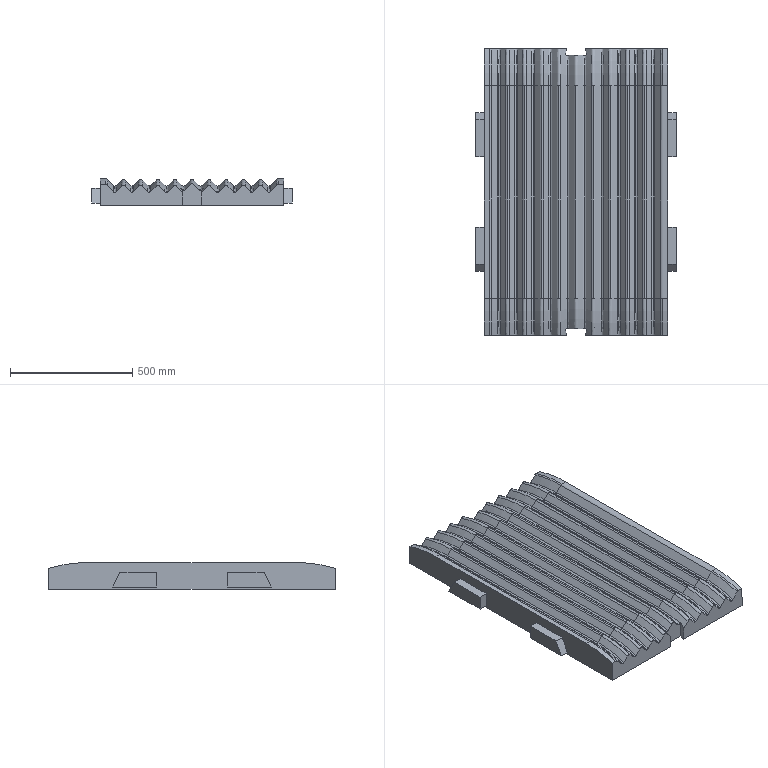Part | SolidWorks | features Fillet 3, ICE 3, LPattern 3, MirrorPattern 2, Extrusion 1, SweepCut 1 | 1 solid | 407 faces | box 820 x 1170 x 110 mm | volume 61269041 mm3 | cylinder 140 | plane 115 | torus 110 | cone 40 | spline 2 | commonest cylinder face diameters 30 x48 60 x48 20 x40 1000 x4